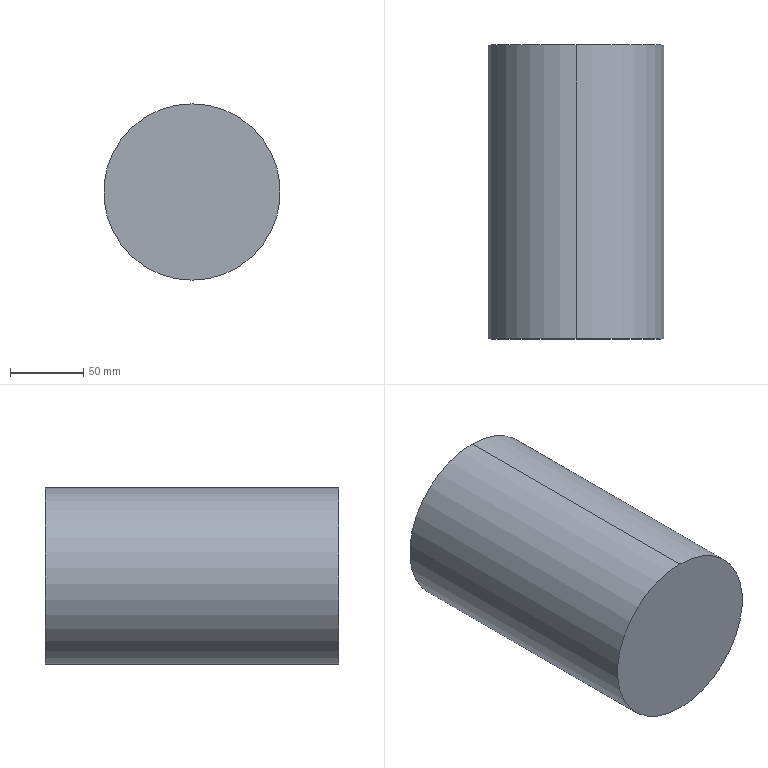Part | SolidWorks | features Extrusion 1, ICE 1 | 1 solid | 7 faces | box 120 x 200 x 120 mm | volume 2249380 mm3 | cylinder 4 | plane 3 | commonest cylinder face diameters 20 x2 120 x2
STEP:
#1=CARTESIAN_POINT('',(0.,160.,-10.));
#2=VERTEX_POINT('',#1);
#3=CARTESIAN_POINT('',(0.,160.,10.));
#4=VERTEX_POINT('',#3);
#5=CARTESIAN_POINT('',(0.,160.,0.));
#6=DIRECTION('',(0.,1.,0.));
#7=DIRECTION('',(0.,0.,1.));
#8=AXIS2_PLACEMENT_3D('',#5,#6,#7);
#9=CIRCLE('',#8,10.);
#10=EDGE_CURVE('',#2,#4,#9,.T.);
#11=ORIENTED_EDGE('',*,*,#10,.F.);
#12=CARTESIAN_POINT('',(0.,200.,-10.));
#13=VERTEX_POINT('',#12);
#14=CARTESIAN_POINT('',(0.,160.,-10.));
#15=DIRECTION('',(0.,1.,0.));
#16=VECTOR('',#15,1000.);
#17=LINE('',#14,#16);
#18=EDGE_CURVE('',#2,#13,#17,.T.);
#19=ORIENTED_EDGE('',*,*,#18,.T.);
#20=CARTESIAN_POINT('',(0.,200.,10.));
#21=VERTEX_POINT('',#20);
#22=CARTESIAN_POINT('',(0.,200.,0.));
#23=DIRECTION('',(0.,1.,0.));
#24=DIRECTION('',(0.,0.,1.));
#25=AXIS2_PLACEMENT_3D('',#22,#23,#24);
#26=CIRCLE('',#25,10.);
#27=EDGE_CURVE('',#13,#21,#26,.T.);
#28=ORIENTED_EDGE('',*,*,#27,.T.);
#29=CARTESIAN_POINT('',(0.,160.,10.));
#30=DIRECTION('',(0.,1.,0.));
#31=VECTOR('',#30,1000.);
#32=LINE('',#29,#31);
#33=EDGE_CURVE('',#4,#21,#32,.T.);
#34=ORIENTED_EDGE('',*,*,#33,.F.);
#35=EDGE_LOOP('',(#11,#19,#28,#34));
#36=FACE_OUTER_BOUND('',#35,.T.);
#37=CARTESIAN_POINT('',(0.,160.,0.));
#38=DIRECTION('',(0.,1.,0.));
#39=DIRECTION('',(0.,0.,1.));
#40=AXIS2_PLACEMENT_3D('',#37,#38,#39);
#41=CYLINDRICAL_SURFACE('',#40,10.);
#42=ADVANCED_FACE('',(#36),#41,.F.);
#43=CARTESIAN_POINT('',(0.,200.,60.));
#44=VERTEX_POINT('',#43);
#45=CARTESIAN_POINT('',(0.,200.,-60.));
#46=VERTEX_POINT('',#45);
#47=CARTESIAN_POINT('',(0.,200.,0.));
#48=DIRECTION('',(0.,1.,0.));
#49=DIRECTION('',(0.,0.,1.));
#50=AXIS2_PLACEMENT_3D('',#47,#48,#49);
#51=CIRCLE('',#50,60.);
#52=EDGE_CURVE('',#44,#46,#51,.T.);
#53=ORIENTED_EDGE('',*,*,#52,.F.);
#54=CARTESIAN_POINT('',(0.,0.,60.));
#55=VERTEX_POINT('',#54);
#56=CARTESIAN_POINT('',(0.,200.,60.));
#57=DIRECTION('',(0.,-1.,0.));
#58=VECTOR('',#57,1000.);
#59=LINE('',#56,#58);
#60=EDGE_CURVE('',#44,#55,#59,.T.);
#61=ORIENTED_EDGE('',*,*,#60,.T.);
#62=CARTESIAN_POINT('',(0.,0.,-60.));
#63=VERTEX_POINT('',#62);
#64=CARTESIAN_POINT('',(0.,0.,0.));
#65=DIRECTION('',(0.,1.,0.));
#66=DIRECTION('',(0.,0.,1.));
#67=AXIS2_PLACEMENT_3D('',#64,#65,#66);
#68=CIRCLE('',#67,60.);
#69=EDGE_CURVE('',#55,#63,#68,.T.);
#70=ORIENTED_EDGE('',*,*,#69,.T.);
#71=CARTESIAN_POINT('',(0.,200.,-60.));
#72=DIRECTION('',(0.,-1.,0.));
#73=VECTOR('',#72,1000.);
#74=LINE('',#71,#73);
#75=EDGE_CURVE('',#46,#63,#74,.T.);
#76=ORIENTED_EDGE('',*,*,#75,.F.);
#77=EDGE_LOOP('',(#53,#61,#70,#76));
#78=FACE_OUTER_BOUND('',#77,.T.);
#79=CARTESIAN_POINT('',(0.,200.,0.));
#80=DIRECTION('',(0.,-1.,0.));
#81=DIRECTION('',(0.,0.,-1.));
#82=AXIS2_PLACEMENT_3D('',#79,#80,#81);
#83=CYLINDRICAL_SURFACE('',#82,60.);
#84=ADVANCED_FACE('',(#78),#83,.T.);
#85=ORIENTED_EDGE('',*,*,#60,.F.);
#86=CARTESIAN_POINT('',(0.,200.,0.));
#87=DIRECTION('',(0.,1.,0.));
#88=DIRECTION('',(0.,0.,1.));
#89=AXIS2_PLACEMENT_3D('',#86,#87,#88);
#90=CIRCLE('',#89,60.);
#91=EDGE_CURVE('',#46,#44,#90,.T.);
#92=ORIENTED_EDGE('',*,*,#91,.F.);
#93=ORIENTED_EDGE('',*,*,#75,.T.);
#94=CARTESIAN_POINT('',(0.,0.,0.));
#95=DIRECTION('',(0.,1.,0.));
#96=DIRECTION('',(0.,0.,1.));
#97=AXIS2_PLACEMENT_3D('',#94,#95,#96);
#98=CIRCLE('',#97,60.);
#99=EDGE_CURVE('',#63,#55,#98,.T.);
#100=ORIENTED_EDGE('',*,*,#99,.T.);
#101=EDGE_LOOP('',(#85,#92,#93,#100));
#102=FACE_OUTER_BOUND('',#101,.T.);
#103=CARTESIAN_POINT('',(0.,200.,0.));
#104=DIRECTION('',(0.,-1.,0.));
#105=DIRECTION('',(0.,0.,-1.));
#106=AXIS2_PLACEMENT_3D('',#103,#104,#105);
#107=CYLINDRICAL_SURFACE('',#106,60.);
#108=ADVANCED_FACE('',(#102),#107,.T.);
#109=CARTESIAN_POINT('',(0.,200.,0.));
#110=DIRECTION('',(0.,1.,0.));
#111=DIRECTION('',(0.,0.,1.));
#112=AXIS2_PLACEMENT_3D('',#109,#110,#111);
#113=CIRCLE('',#112,10.);
#114=EDGE_CURVE('',#21,#13,#113,.T.);
#115=ORIENTED_EDGE('',*,*,#114,.F.);
#116=ORIENTED_EDGE('',*,*,#27,.F.);
#117=EDGE_LOOP('',(#115,#116));
#118=FACE_BOUND('',#117,.T.);
#119=ORIENTED_EDGE('',*,*,#91,.T.);
#120=ORIENTED_EDGE('',*,*,#52,.T.);
#121=EDGE_LOOP('',(#119,#120));
#122=FACE_OUTER_BOUND('',#121,.T.);
#123=CARTESIAN_POINT('',(0.,200.,0.));
#124=DIRECTION('',(0.,1.,0.));
#125=DIRECTION('',(0.,0.,1.));
#126=AXIS2_PLACEMENT_3D('',#123,#124,#125);
#127=PLANE('',#126);
#128=ADVANCED_FACE('',(#118,#122),#127,.T.);
#129=ORIENTED_EDGE('',*,*,#99,.F.);
#130=ORIENTED_EDGE('',*,*,#69,.F.);
#131=EDGE_LOOP('',(#129,#130));
#132=FACE_OUTER_BOUND('',#131,.T.);
#133=CARTESIAN_POINT('',(0.,0.,0.));
#134=DIRECTION('',(0.,1.,0.));
#135=DIRECTION('',(0.,0.,1.));
#136=AXIS2_PLACEMENT_3D('',#133,#134,#135);
#137=PLANE('',#136);
#138=ADVANCED_FACE('',(#132),#137,.F.);
#139=ORIENTED_EDGE('',*,*,#18,.F.);
#140=CARTESIAN_POINT('',(0.,160.,0.));
#141=DIRECTION('',(0.,1.,0.));
#142=DIRECTION('',(0.,0.,1.));
#143=AXIS2_PLACEMENT_3D('',#140,#141,#142);
#144=CIRCLE('',#143,10.);
#145=EDGE_CURVE('',#4,#2,#144,.T.);
#146=ORIENTED_EDGE('',*,*,#145,.F.);
#147=ORIENTED_EDGE('',*,*,#33,.T.);
#148=ORIENTED_EDGE('',*,*,#114,.T.);
#149=EDGE_LOOP('',(#139,#146,#147,#148));
#150=FACE_OUTER_BOUND('',#149,.T.);
#151=CARTESIAN_POINT('',(0.,160.,0.));
#152=DIRECTION('',(0.,1.,0.));
#153=DIRECTION('',(0.,0.,1.));
#154=AXIS2_PLACEMENT_3D('',#151,#152,#153);
#155=CYLINDRICAL_SURFACE('',#154,10.);
#156=ADVANCED_FACE('',(#150),#155,.F.);
#157=ORIENTED_EDGE('',*,*,#145,.T.);
#158=ORIENTED_EDGE('',*,*,#10,.T.);
#159=EDGE_LOOP('',(#157,#158));
#160=FACE_OUTER_BOUND('',#159,.T.);
#161=CARTESIAN_POINT('',(0.,160.,0.));
#162=DIRECTION('',(0.,1.,0.));
#163=DIRECTION('',(0.,0.,1.));
#164=AXIS2_PLACEMENT_3D('',#161,#162,#163);
#165=PLANE('',#164);
#166=ADVANCED_FACE('',(#160),#165,.T.);
#167=CLOSED_SHELL('',(#42,#84,#108,#128,#138,#156,#166));
#168=MANIFOLD_SOLID_BREP('',#167);
#169=CARTESIAN_POINT('',(0.,0.,0.));
#170=DIRECTION('',(0.,0.,1.));
#171=DIRECTION('',(1.,0.,0.));
#172=AXIS2_PLACEMENT_3D('',#169,#170,#171);
#173=(LENGTH_UNIT()NAMED_UNIT(*)SI_UNIT(.MILLI.,.METRE.));
#174=UNCERTAINTY_MEASURE_WITH_UNIT(LENGTH_MEASURE(0.00001),#173,'','');
#175=(NAMED_UNIT(*)PLANE_ANGLE_UNIT()SI_UNIT($,.RADIAN.));
#176=(NAMED_UNIT(*)SI_UNIT($,.STERADIAN.)SOLID_ANGLE_UNIT());
#177=(GEOMETRIC_REPRESENTATION_CONTEXT(3)GLOBAL_UNCERTAINTY_ASSIGNED_CONTEXT((#174))GLOBAL_UNIT_ASSIGNED_CONTEXT((#173,#175,#176))REPRESENTATION_CONTEXT('',''));
#178=ADVANCED_BREP_SHAPE_REPRESENTATION('',(#168,#172),#177);